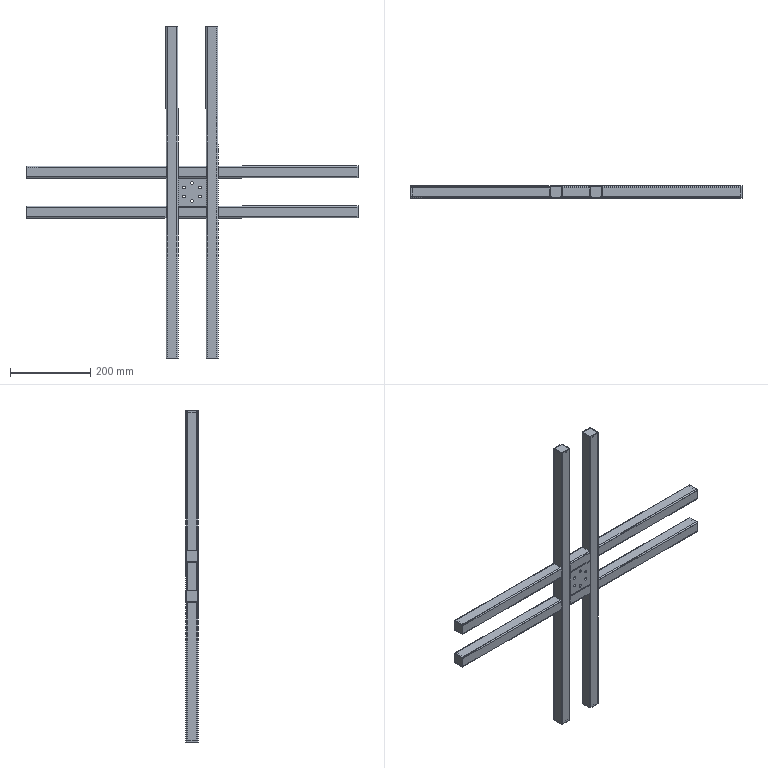Part | SolidWorks | 17 solids | 242 faces | box 830 x 30 x 830 mm | volume 603556 mm3 | plane 134 | cylinder 108 | commonest cylinder face diameters 6 x64 3 x32 7 x12